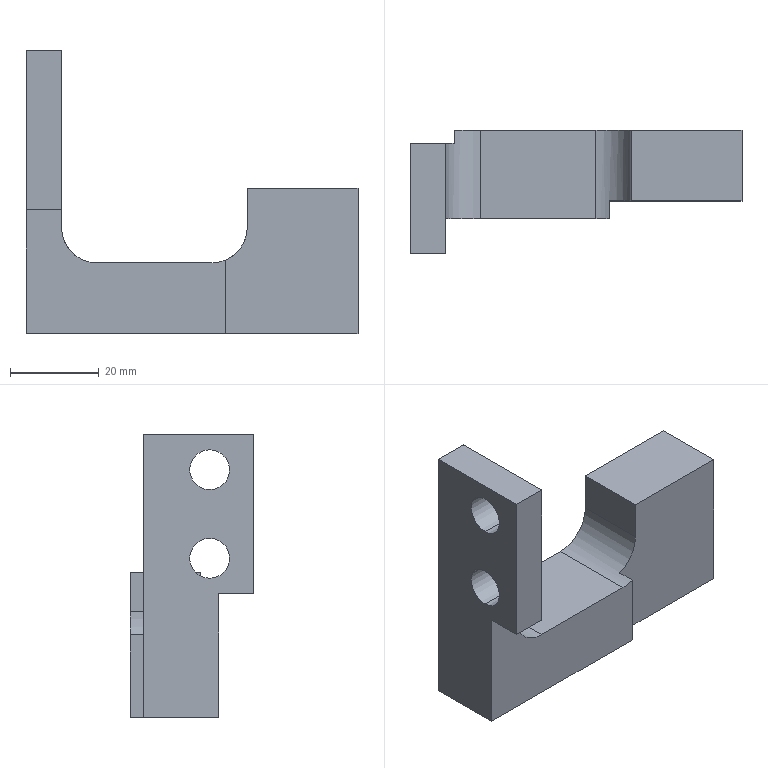Part | STEP file | OP10-159_seal block (2nd air pass) | 1 solid | 32 faces | box 75 x 28 x 64 mm | volume 36277 mm3 | plane 18 | cylinder 12 | cone 2 | commonest cylinder face diameters 9 x4 3.3 x2 6 x2 11 x2 16 x2